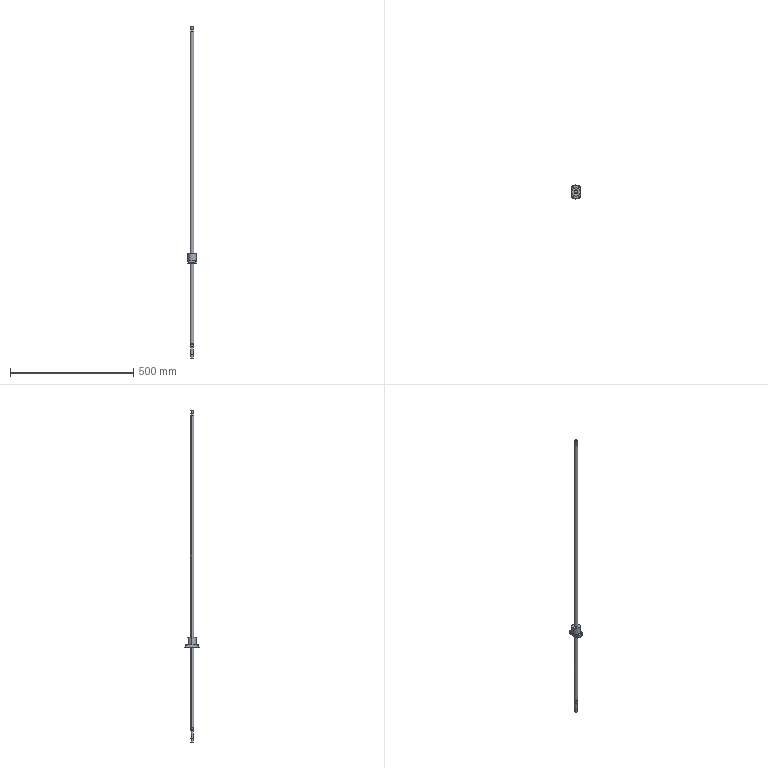Part | STEP file | r14-5b1-fsw150-2 | 1 solid | 65 faces | box 34 x 57 x 1346 mm | volume 239827 mm3 | cylinder 38 | plane 27 | commonest cylinder face diameters 5.5 x8 9.5 x8 10 x6 14 x4 9.6 x2 10.5 x2